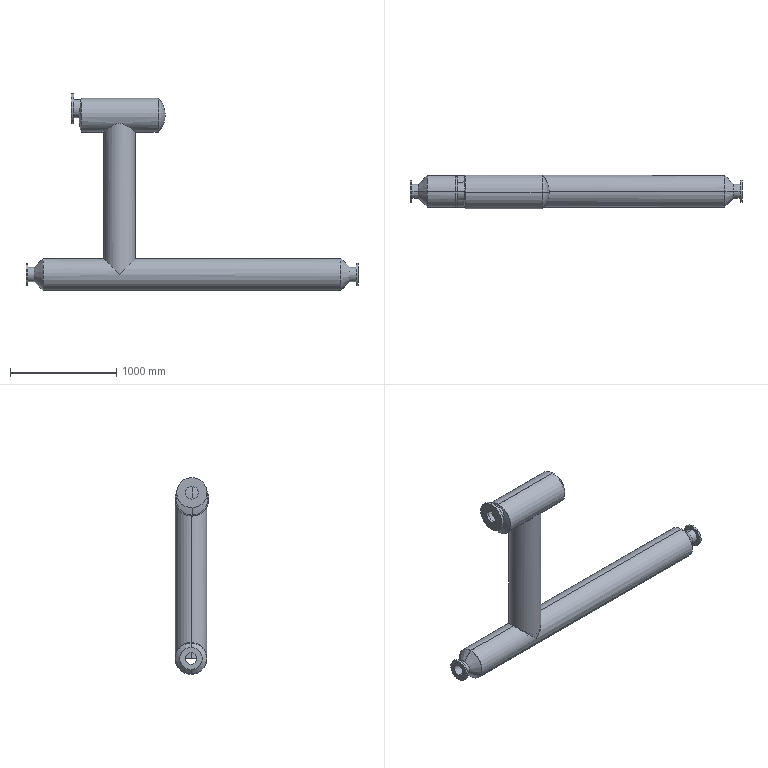Part | SolidWorks | features ICE 3, Revolution 2 | 1 solid | 85 faces | box 3124 x 319.547 x 1852 mm | volume 52039073 mm3 | cylinder 54 | torus 12 | plane 11 | cone 8 | commonest cylinder face diameters 280 x12 300 x12 113 x4 133 x4 150 x4 170 x4